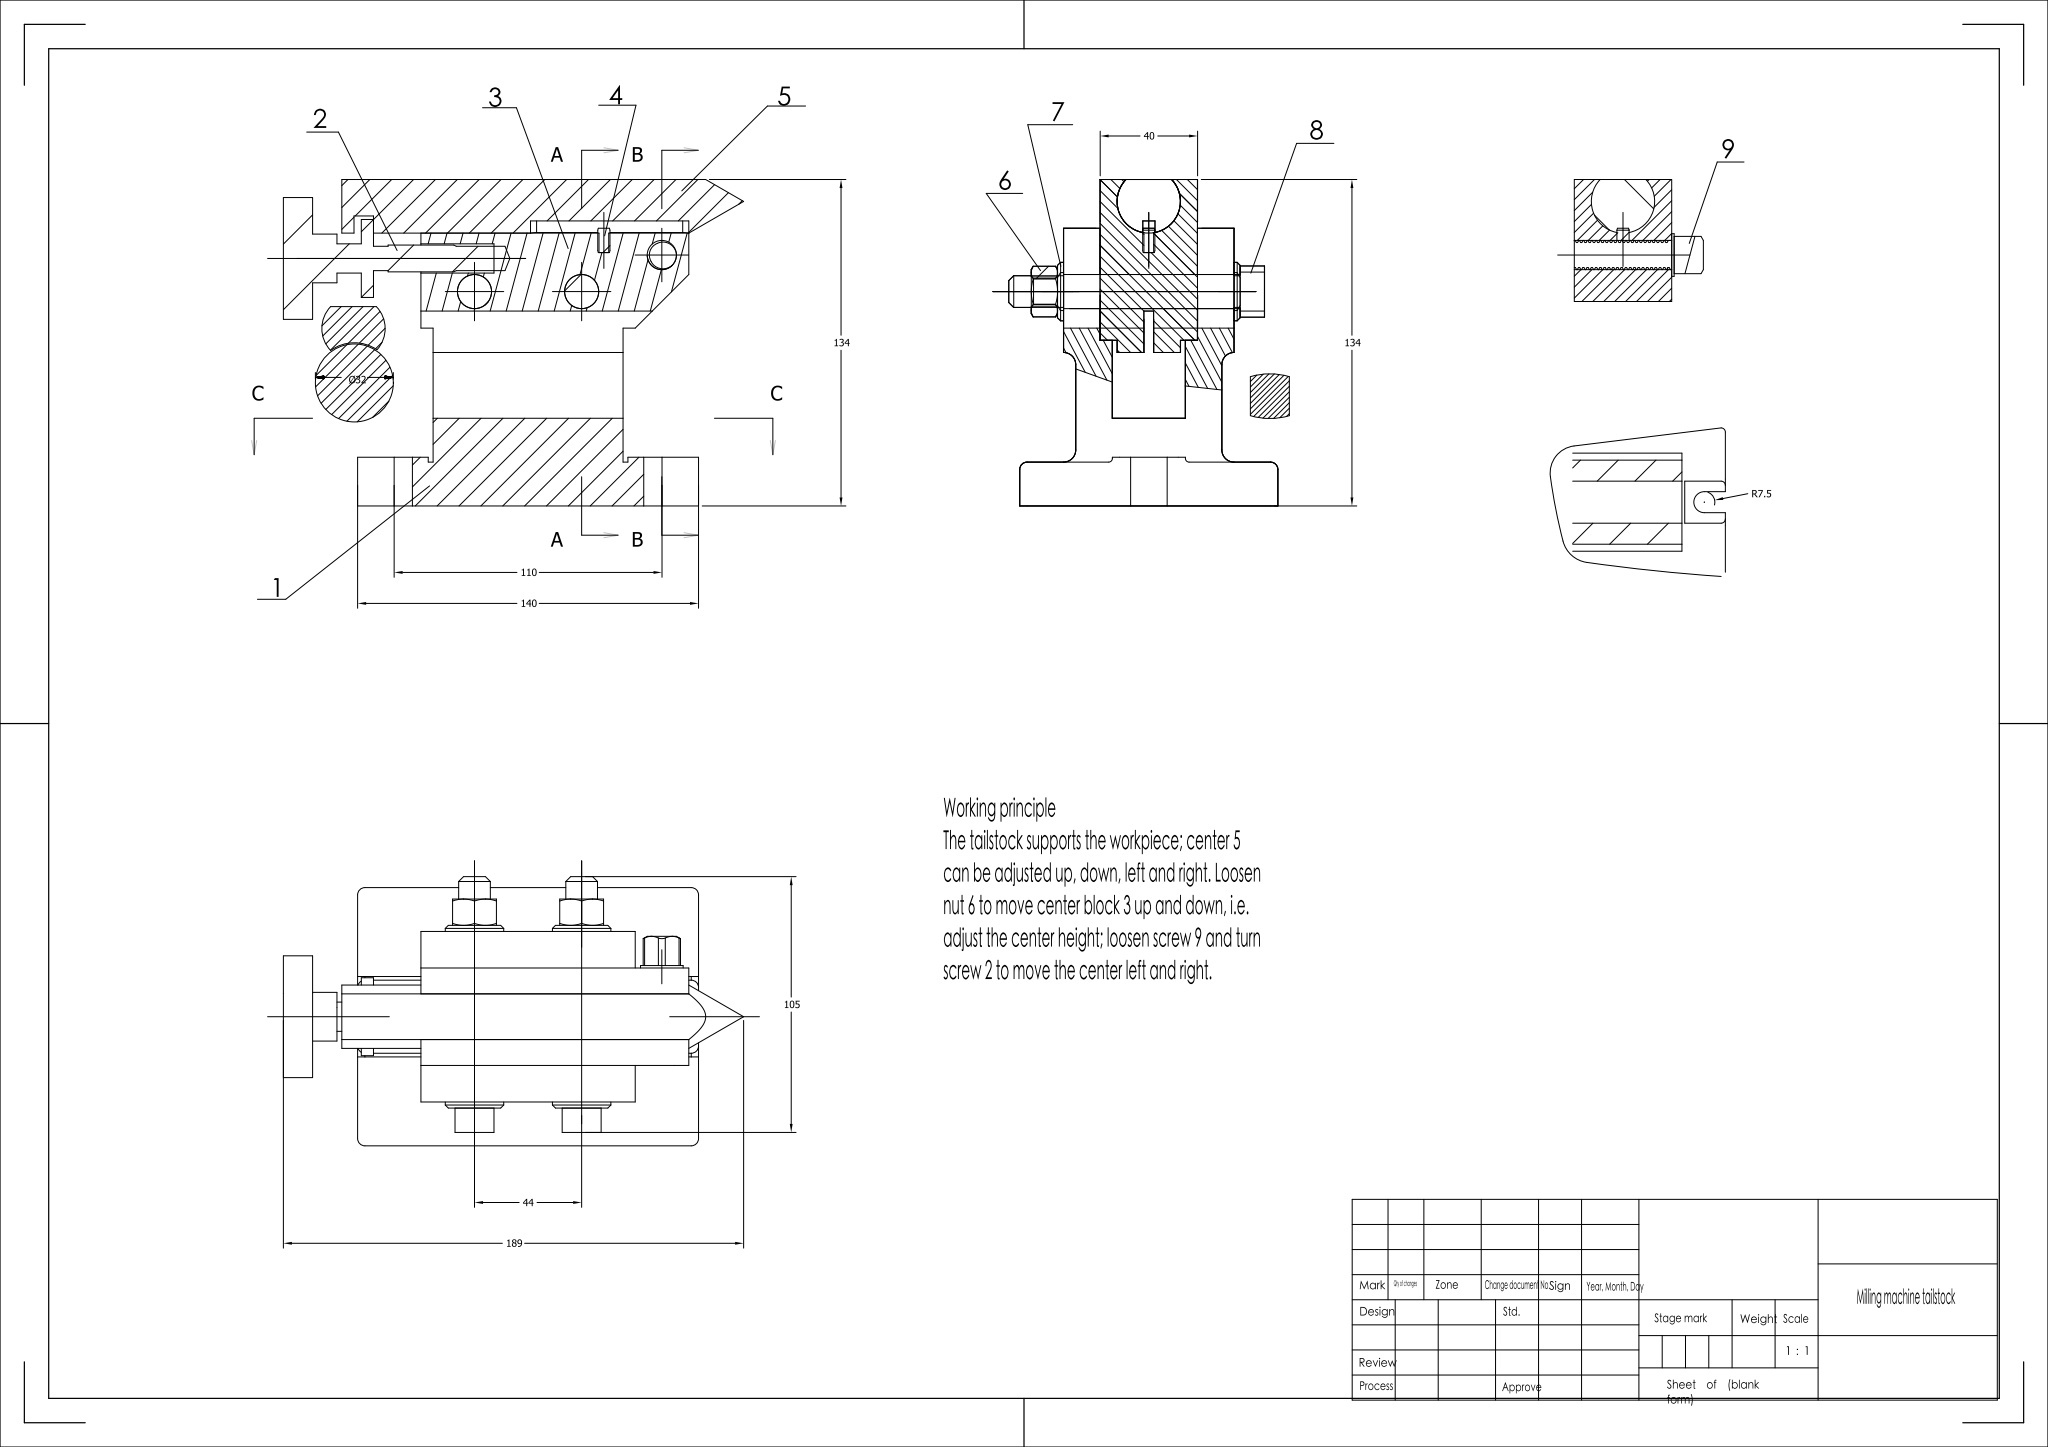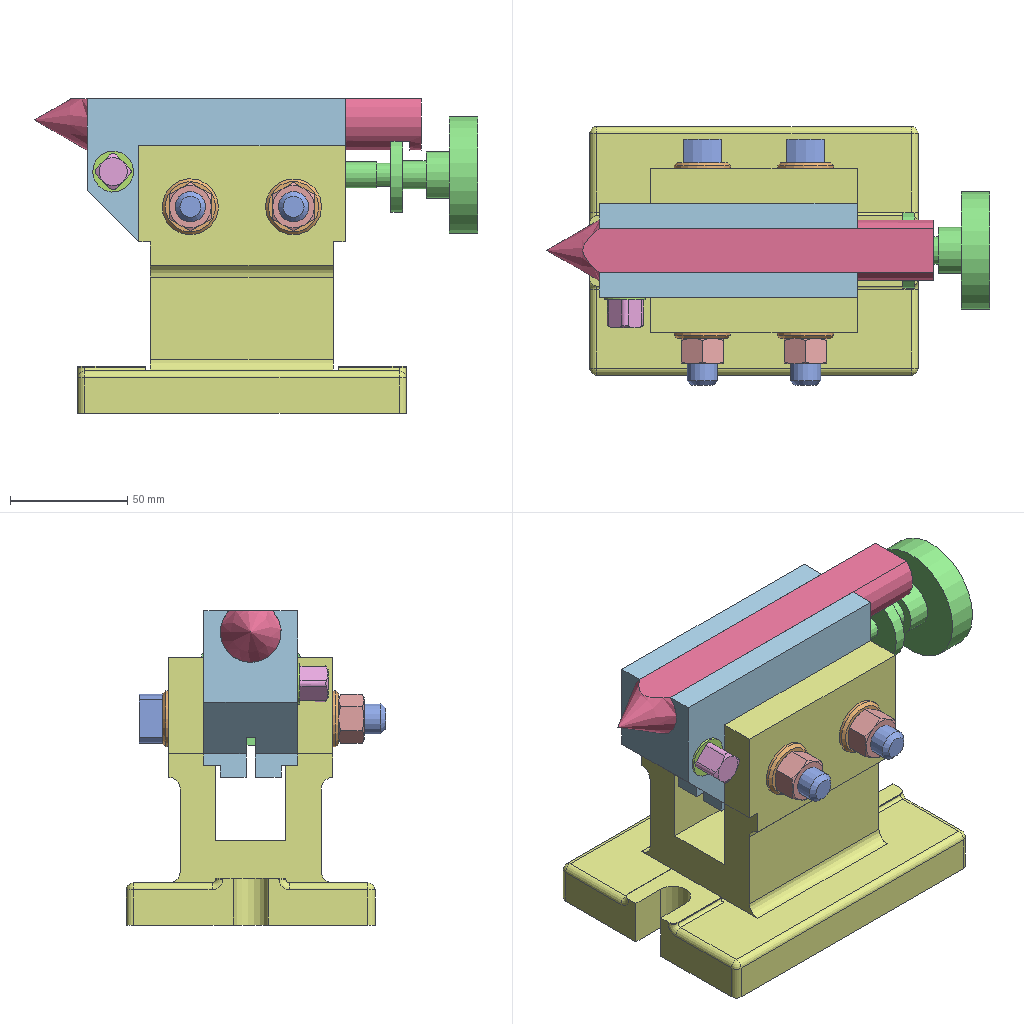Assembly | NX | 9 different items | 14 placed | box 189 x 111 x 134 mm
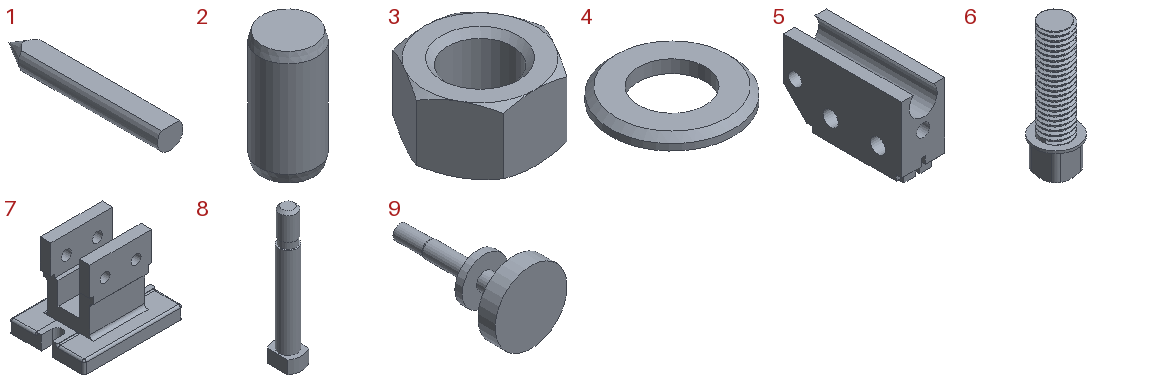Parts list (item | quantity | size | volume | features):
1 | x1 | 26 x 165 x 22 mm | 69817 mm3 | features EXTRUDE 4, DATUM_CSYS 2, CONE 1, DATUM_PLANE 1, RECT_SLOT 1, SKETCH 1
2 | x1 | 5 x 5 x 10 mm | 193.733 mm3 | features DATUM_CSYS 2, LINE 1, SKETCH 1, SWP104 1
3 | x2 | 20.785 x 18 x 10.8 mm | 2032 mm3 | features META 3, SKETCH 3, DATUM_CSYS 2, EXTRUDE 2, SWP104 2, CHAMFER 1, LINE 1, SYMBOLIC_THREAD 1, THREADS 1
4 | x4 | 24 x 24 x 2.5 mm | 742.283 mm3 | features DATUM_CSYS 2, CHAMFER 1, EXTRUDE 1, LINE 1, SKETCH 1
5 | x1 | 40 x 110 x 71 mm | 205746 mm3 | features EXTRUDE 7, DATUM_CSYS 6, SKETCH 5
6 | x1 | 17.5 x 17.5 x 53 mm | 5763 mm3 | features EXTRUDE 4, DATUM_CSYS 2, SKETCH 1, THREADS 1
7 | x1 | 140 x 106 x 114 mm | 532545 mm3 | features EXTRUDE 8, FACE_BLEND 6, DATUM_CSYS 5, SKETCH 4, BLEND 1
8 | x2 | 16 x 21.022 x 105 mm | 17029 mm3 | features EXTRUDE 4, DATUM_CSYS 2, CHAMFER 1, SKETCH 1
9 | x1 | 50 x 93 x 50 mm | 36603 mm3 | features EXTRUDE 7, DATUM_CSYS 5, SKETCH 4, CONE 2, UNITE 1
Mates (type | each side: item.copy, entity, surface, feature):
Touch | 5.1 face cylinder Extrude(5) | 7.1 face cylinder Extrude(15)
Touch | 5.1 face plane Extrude(2) | 7.1 face plane Extrude(6)
Touch | 1.1 face cylinder Extrude(2) | 5.1 face cylinder Extrude(2)
Parallel | 1.1 face plane Extrude(2) | 7.1 face plane Extrude(18)
Concentric | 1.1 edge | 5.1 edge
Touch | 9.1 face cylinder Extrude(10) | 5.1 face cylinder Extrude(4)
Touch | 9.1 face plane Extrude(3) | 1.1 face plane Extrude(3)
Touch | 2.1 face cylinder Revolve(16) | 5.1 face cylinder Extrude(12)
Concentric | 2.1 edge | 5.1 edge
Touch | 4.1 face cylinder Extrude(16) | 7.1 face cylinder Extrude(16)
Touch | 4.1 face plane Extrude(16) | 7.1 face plane Extrude(6) | 4 times
Touch | 4.1 face cone Chamfer(19) | 7.1 face cylinder Extrude(16)
Touch | 4.1 face cone Chamfer(19) | 7.1 face cylinder Extrude(15)
Touch | 4.1 face cylinder Extrude(16) | 7.1 face cylinder Extrude(15)
Touch | 6.1 face cylinder Threads(6) | 5.1 face cylinder Extrude(13)
Touch | 6.1 face plane Extrude(4) | 5.1 face plane Extrude(2)
Angle | 6.1 face plane Extrude(3) | 7.1 face plane Extrude(19)
Touch | 8.1 face cylinder Extrude(8) | 7.1 face cylinder Extrude(15) | 2 times
Touch | 8.1 face plane Extrude(7) | 4.1 face plane Extrude(16) | 2 times
Parallel | 8.1 edge | 7.1 edge | 2 times
Touch | 3.1 face cylinder Extrude(6) | 8.1 face cylinder Extrude(10) | 2 times
Touch | 3.1 face plane Extrude(5) | 4.1 face plane Extrude(16) | 2 times
Parallel | 3.1 face plane Extrude(5) | 7.1 face plane Extrude(19) | 2 times